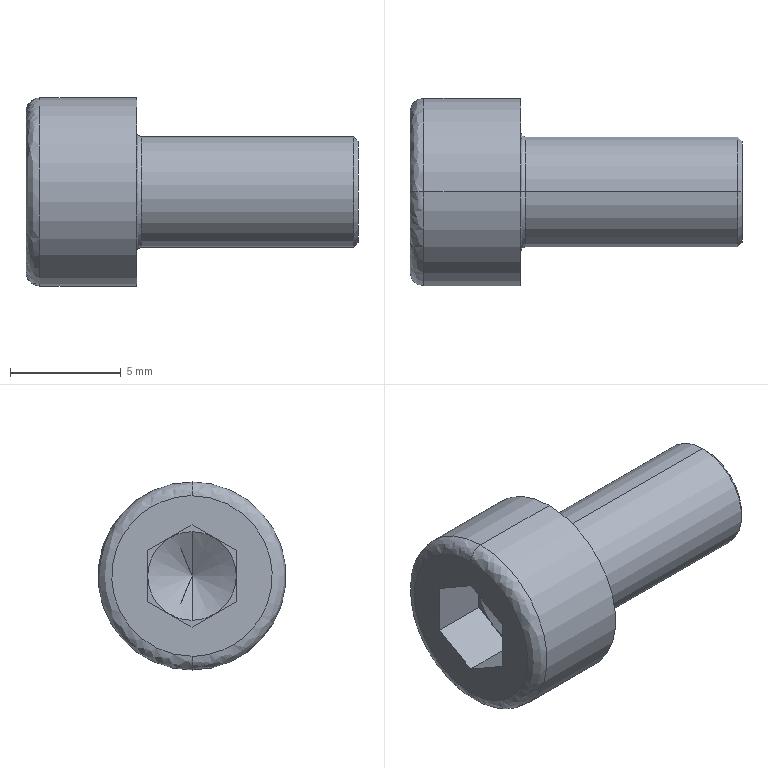Part | SolidWorks | features BaseBody 1 | 1 solid | 27 faces | box 15 x 8.5 x 8.5 mm | volume 438.278 mm3 | plane 15 | spline 4 | cylinder 4 | cone 4 | commonest cylinder face diameters 5 x2 8.5 x2
STEP:
#1=CARTESIAN_POINT('',(5.,0.,2.7));
#2=VERTEX_POINT('',#1);
#3=CARTESIAN_POINT('',(5.,0.,-2.7));
#4=VERTEX_POINT('',#3);
#5=CARTESIAN_POINT('',(5.,0.,2.7));
#6=CARTESIAN_POINT('',(5.,0.1716,2.7));
#7=CARTESIAN_POINT('',(5.,0.4245,2.676));
#8=CARTESIAN_POINT('',(5.,0.7118,2.607));
#9=CARTESIAN_POINT('',(5.,0.8535,2.562));
#10=CARTESIAN_POINT('',(5.,0.9138,2.541));
#11=CARTESIAN_POINT('',(5.,0.9539,2.526));
#12=CARTESIAN_POINT('',(5.,0.9722,2.519));
#13=CARTESIAN_POINT('',(5.,1.34,2.373));
#14=CARTESIAN_POINT('',(5.,1.646,2.172));
#15=CARTESIAN_POINT('',(5.,2.041,1.778));
#16=CARTESIAN_POINT('',(5.,2.215,1.564));
#17=CARTESIAN_POINT('',(5.,2.376,1.288));
#18=CARTESIAN_POINT('',(5.,2.447,1.143));
#19=CARTESIAN_POINT('',(5.,2.475,1.08));
#20=CARTESIAN_POINT('',(5.,2.493,1.037));
#21=CARTESIAN_POINT('',(5.,2.503,1.014));
#22=CARTESIAN_POINT('',(5.,2.637,0.675));
#23=CARTESIAN_POINT('',(5.,2.7,0.343));
#24=CARTESIAN_POINT('',(5.,2.7,-0.1715));
#25=CARTESIAN_POINT('',(5.,2.676,-0.4243));
#26=CARTESIAN_POINT('',(5.,2.607,-0.7117));
#27=CARTESIAN_POINT('',(5.,2.562,-0.8534));
#28=CARTESIAN_POINT('',(5.,2.541,-0.9137));
#29=CARTESIAN_POINT('',(5.,2.526,-0.9539));
#30=CARTESIAN_POINT('',(5.,2.519,-0.9722));
#31=CARTESIAN_POINT('',(5.,2.373,-1.34));
#32=CARTESIAN_POINT('',(5.,2.172,-1.646));
#33=CARTESIAN_POINT('',(5.,1.778,-2.041));
#34=CARTESIAN_POINT('',(5.,1.564,-2.215));
#35=CARTESIAN_POINT('',(5.,1.288,-2.376));
#36=CARTESIAN_POINT('',(5.,1.143,-2.447));
#37=CARTESIAN_POINT('',(5.,1.08,-2.475));
#38=CARTESIAN_POINT('',(5.,1.037,-2.493));
#39=CARTESIAN_POINT('',(5.,1.014,-2.503));
#40=CARTESIAN_POINT('',(5.,0.6748,-2.637));
#41=CARTESIAN_POINT('',(5.,0.3435,-2.7));
#42=CARTESIAN_POINT('',(5.,0.,-2.7));
#43=B_SPLINE_CURVE_WITH_KNOTS('',3,(#5,#6,#7,#8,#9,#10,#11,#12,#13,#14,#15,#16,#17,#18,#19,#20,#21,#22,#23,#24,#25,#26,#27,#28,#29,#30,#31,#32,#33,#34,#35,#36,#37,#38,#39,#40,#41,#42),.UNSPECIFIED.,.F.,.F.,(4,1,1,1,2,2,2,1,1,1,2,2,2,1,1,1,2,2,2,1,1,1,2,2,4),(0.,0.0625,0.09375,0.1094,0.1172,0.125,0.25,0.3125,0.3437,0.3594,0.3672,0.375,0.5,0.5625,0.5937,0.6094,0.6172,0.625,0.75,0.8125,0.8437,0.8594,0.8672,0.875,1.),.UNSPECIFIED.);
#44=EDGE_CURVE('',#2,#4,#43,.T.);
#45=ORIENTED_EDGE('',*,*,#44,.F.);
#46=CARTESIAN_POINT('',(5.2,0.,2.5));
#47=VERTEX_POINT('',#46);
#48=CARTESIAN_POINT('',(5.2,0.,2.7));
#49=DIRECTION('',(0.,-1.,0.));
#50=DIRECTION('',(0.,0.,1.));
#51=AXIS2_PLACEMENT_3D('',#48,#49,#50);
#52=CIRCLE('',#51,0.2);
#53=EDGE_CURVE('',#2,#47,#52,.T.);
#54=ORIENTED_EDGE('',*,*,#53,.T.);
#55=CARTESIAN_POINT('',(5.2,0.,-2.5));
#56=VERTEX_POINT('',#55);
#57=CARTESIAN_POINT('',(5.2,0.,0.));
#58=DIRECTION('',(1.,0.,0.));
#59=DIRECTION('',(0.,0.,1.));
#60=AXIS2_PLACEMENT_3D('',#57,#58,#59);
#61=CIRCLE('',#60,2.5);
#62=EDGE_CURVE('',#56,#47,#61,.T.);
#63=ORIENTED_EDGE('',*,*,#62,.F.);
#64=CARTESIAN_POINT('',(5.2,0.,-2.7));
#65=DIRECTION('',(0.,1.,0.));
#66=DIRECTION('',(0.,0.,-1.));
#67=AXIS2_PLACEMENT_3D('',#64,#65,#66);
#68=CIRCLE('',#67,0.2);
#69=EDGE_CURVE('',#4,#56,#68,.T.);
#70=ORIENTED_EDGE('',*,*,#69,.F.);
#71=EDGE_LOOP('',(#45,#54,#63,#70));
#72=FACE_OUTER_BOUND('',#71,.T.);
#73=CARTESIAN_POINT('',(5.,0.,-2.7));
#74=CARTESIAN_POINT('',(5.,5.4,-2.7));
#75=CARTESIAN_POINT('',(5.,5.4,2.7));
#76=CARTESIAN_POINT('',(5.,0.,2.7));
#77=CARTESIAN_POINT('',(5.,0.,-2.583));
#78=CARTESIAN_POINT('',(5.,5.166,-2.583));
#79=CARTESIAN_POINT('',(5.,5.166,2.583));
#80=CARTESIAN_POINT('',(5.,0.,2.583));
#81=CARTESIAN_POINT('',(5.083,0.,-2.5));
#82=CARTESIAN_POINT('',(5.083,5.,-2.5));
#83=CARTESIAN_POINT('',(5.083,5.,2.5));
#84=CARTESIAN_POINT('',(5.083,0.,2.5));
#85=CARTESIAN_POINT('',(5.2,0.,-2.5));
#86=CARTESIAN_POINT('',(5.2,5.,-2.5));
#87=CARTESIAN_POINT('',(5.2,5.,2.5));
#88=CARTESIAN_POINT('',(5.2,0.,2.5));
#89=(BOUNDED_SURFACE()B_SPLINE_SURFACE(3,3,((#73,#74,#75,#76),(#77,#78,#79,#80),(#81,#82,#83,#84),(#85,#86,#87,#88)),.UNSPECIFIED.,.F.,.F.,.F.)B_SPLINE_SURFACE_WITH_KNOTS((4,4),(4,4),(0.,1.),(0.,1.),.UNSPECIFIED.)GEOMETRIC_REPRESENTATION_ITEM()RATIONAL_B_SPLINE_SURFACE(((1.,0.3333,0.3333,1.),(0.8047,0.2682,0.2682,0.8047),(0.8047,0.2682,0.2682,0.8047),(1.,0.3333,0.3333,1.)))REPRESENTATION_ITEM('')SURFACE());
#90=ADVANCED_FACE('',(#72),#89,.F.);
#91=CARTESIAN_POINT('',(0.625,0.,4.25));
#92=VERTEX_POINT('',#91);
#93=CARTESIAN_POINT('',(0.625,0.,-4.25));
#94=VERTEX_POINT('',#93);
#95=CARTESIAN_POINT('',(0.625,0.,0.));
#96=DIRECTION('',(1.,0.,0.));
#97=DIRECTION('',(0.,0.,1.));
#98=AXIS2_PLACEMENT_3D('',#95,#96,#97);
#99=CIRCLE('',#98,4.25);
#100=EDGE_CURVE('',#92,#94,#99,.T.);
#101=ORIENTED_EDGE('',*,*,#100,.F.);
#102=CARTESIAN_POINT('',(0.,0.,3.625));
#103=VERTEX_POINT('',#102);
#104=CARTESIAN_POINT('',(0.625,0.,3.625));
#105=DIRECTION('',(0.,-1.,0.));
#106=DIRECTION('',(0.,0.,1.));
#107=AXIS2_PLACEMENT_3D('',#104,#105,#106);
#108=CIRCLE('',#107,0.625);
#109=EDGE_CURVE('',#92,#103,#108,.T.);
#110=ORIENTED_EDGE('',*,*,#109,.T.);
#111=CARTESIAN_POINT('',(0.,0.,-3.625));
#112=VERTEX_POINT('',#111);
#113=CARTESIAN_POINT('',(0.,0.,3.625));
#114=CARTESIAN_POINT('',(0.,-7.25,3.625));
#115=CARTESIAN_POINT('',(0.,-7.25,-3.625));
#116=CARTESIAN_POINT('',(0.,0.,-3.625));
#117=(BOUNDED_CURVE()B_SPLINE_CURVE(3,(#113,#114,#115,#116),.UNSPECIFIED.,.F.,.F.)B_SPLINE_CURVE_WITH_KNOTS((4,4),(0.,1.),.UNSPECIFIED.)CURVE()GEOMETRIC_REPRESENTATION_ITEM()RATIONAL_B_SPLINE_CURVE((1.,0.3333,0.3333,1.))REPRESENTATION_ITEM(''));
#118=EDGE_CURVE('',#103,#112,#117,.T.);
#119=ORIENTED_EDGE('',*,*,#118,.T.);
#120=CARTESIAN_POINT('',(0.625,0.,-3.625));
#121=DIRECTION('',(0.,1.,0.));
#122=DIRECTION('',(0.,0.,-1.));
#123=AXIS2_PLACEMENT_3D('',#120,#121,#122);
#124=CIRCLE('',#123,0.625);
#125=EDGE_CURVE('',#94,#112,#124,.T.);
#126=ORIENTED_EDGE('',*,*,#125,.F.);
#127=EDGE_LOOP('',(#101,#110,#119,#126));
#128=FACE_OUTER_BOUND('',#127,.T.);
#129=CARTESIAN_POINT('',(0.625,0.,4.25));
#130=CARTESIAN_POINT('',(0.625,-8.5,4.25));
#131=CARTESIAN_POINT('',(0.625,-8.5,-4.25));
#132=CARTESIAN_POINT('',(0.625,0.,-4.25));
#133=CARTESIAN_POINT('',(0.2589,0.,4.25));
#134=CARTESIAN_POINT('',(0.2589,-8.5,4.25));
#135=CARTESIAN_POINT('',(0.2589,-8.5,-4.25));
#136=CARTESIAN_POINT('',(0.2589,0.,-4.25));
#137=CARTESIAN_POINT('',(0.,0.,3.991));
#138=CARTESIAN_POINT('',(0.,-7.982,3.991));
#139=CARTESIAN_POINT('',(0.,-7.982,-3.991));
#140=CARTESIAN_POINT('',(0.,0.,-3.991));
#141=CARTESIAN_POINT('',(0.,0.,3.625));
#142=CARTESIAN_POINT('',(0.,-7.25,3.625));
#143=CARTESIAN_POINT('',(0.,-7.25,-3.625));
#144=CARTESIAN_POINT('',(0.,0.,-3.625));
#145=(BOUNDED_SURFACE()B_SPLINE_SURFACE(3,3,((#129,#130,#131,#132),(#133,#134,#135,#136),(#137,#138,#139,#140),(#141,#142,#143,#144)),.UNSPECIFIED.,.F.,.F.,.F.)B_SPLINE_SURFACE_WITH_KNOTS((4,4),(4,4),(0.,1.),(0.,1.),.UNSPECIFIED.)GEOMETRIC_REPRESENTATION_ITEM()RATIONAL_B_SPLINE_SURFACE(((1.,0.3333,0.3333,1.),(0.8047,0.2682,0.2682,0.8047),(0.8047,0.2682,0.2682,0.8047),(1.,0.3333,0.3333,1.)))REPRESENTATION_ITEM('')SURFACE());
#146=ADVANCED_FACE('',(#128),#145,.T.);
#147=CARTESIAN_POINT('',(14.8,0.,2.5));
#148=VERTEX_POINT('',#147);
#149=CARTESIAN_POINT('',(14.8,0.,-2.5));
#150=VERTEX_POINT('',#149);
#151=CARTESIAN_POINT('',(14.8,0.,0.));
#152=DIRECTION('',(-1.,0.,0.));
#153=DIRECTION('',(0.,0.,1.));
#154=AXIS2_PLACEMENT_3D('',#151,#152,#153);
#155=CIRCLE('',#154,2.5);
#156=EDGE_CURVE('',#148,#150,#155,.T.);
#157=ORIENTED_EDGE('',*,*,#156,.T.);
#158=CARTESIAN_POINT('',(15.,0.,-2.5));
#159=DIRECTION('',(-1.,0.,0.));
#160=VECTOR('',#159,1000.);
#161=LINE('',#158,#160);
#162=EDGE_CURVE('',#150,#56,#161,.T.);
#163=ORIENTED_EDGE('',*,*,#162,.T.);
#164=ORIENTED_EDGE('',*,*,#62,.T.);
#165=CARTESIAN_POINT('',(15.,0.,2.5));
#166=DIRECTION('',(-1.,0.,0.));
#167=VECTOR('',#166,1000.);
#168=LINE('',#165,#167);
#169=EDGE_CURVE('',#148,#47,#168,.T.);
#170=ORIENTED_EDGE('',*,*,#169,.F.);
#171=EDGE_LOOP('',(#157,#163,#164,#170));
#172=FACE_OUTER_BOUND('',#171,.T.);
#173=CARTESIAN_POINT('',(15.,0.,0.));
#174=DIRECTION('',(-1.,0.,0.));
#175=DIRECTION('',(0.,0.,1.));
#176=AXIS2_PLACEMENT_3D('',#173,#174,#175);
#177=CYLINDRICAL_SURFACE('',#176,2.5);
#178=ADVANCED_FACE('',(#172),#177,.T.);
#179=CARTESIAN_POINT('',(15.,0.,2.3));
#180=VERTEX_POINT('',#179);
#181=CARTESIAN_POINT('',(15.,0.,-2.3));
#182=VERTEX_POINT('',#181);
#183=CARTESIAN_POINT('',(15.,0.,0.));
#184=DIRECTION('',(-1.,0.,0.));
#185=DIRECTION('',(0.,0.,1.));
#186=AXIS2_PLACEMENT_3D('',#183,#184,#185);
#187=CIRCLE('',#186,2.3);
#188=EDGE_CURVE('',#180,#182,#187,.T.);
#189=ORIENTED_EDGE('',*,*,#188,.T.);
#190=CARTESIAN_POINT('',(14.8,0.,-2.5));
#191=DIRECTION('',(-0.7071,0.,-0.7071));
#192=VECTOR('',#191,1000.);
#193=LINE('',#190,#192);
#194=EDGE_CURVE('',#182,#150,#193,.T.);
#195=ORIENTED_EDGE('',*,*,#194,.T.);
#196=ORIENTED_EDGE('',*,*,#156,.F.);
#197=CARTESIAN_POINT('',(14.8,0.,2.5));
#198=DIRECTION('',(-0.7071,0.,0.7071));
#199=VECTOR('',#198,1000.);
#200=LINE('',#197,#199);
#201=EDGE_CURVE('',#180,#148,#200,.T.);
#202=ORIENTED_EDGE('',*,*,#201,.F.);
#203=EDGE_LOOP('',(#189,#195,#196,#202));
#204=FACE_OUTER_BOUND('',#203,.T.);
#205=CARTESIAN_POINT('',(14.8,0.,0.));
#206=DIRECTION('',(-1.,0.,0.));
#207=DIRECTION('',(0.,0.,1.));
#208=AXIS2_PLACEMENT_3D('',#205,#206,#207);
#209=CONICAL_SURFACE('',#208,2.5,0.7854);
#210=ADVANCED_FACE('',(#204),#209,.T.);
#211=CARTESIAN_POINT('',(5.,0.,-4.25));
#212=VERTEX_POINT('',#211);
#213=CARTESIAN_POINT('',(5.,0.,4.25));
#214=VERTEX_POINT('',#213);
#215=CARTESIAN_POINT('',(5.,0.,0.));
#216=DIRECTION('',(1.,0.,0.));
#217=DIRECTION('',(0.,0.,1.));
#218=AXIS2_PLACEMENT_3D('',#215,#216,#217);
#219=CIRCLE('',#218,4.25);
#220=EDGE_CURVE('',#212,#214,#219,.T.);
#221=ORIENTED_EDGE('',*,*,#220,.F.);
#222=CARTESIAN_POINT('',(5.,0.,-4.25));
#223=DIRECTION('',(-1.,0.,0.));
#224=VECTOR('',#223,1000.);
#225=LINE('',#222,#224);
#226=EDGE_CURVE('',#212,#94,#225,.T.);
#227=ORIENTED_EDGE('',*,*,#226,.T.);
#228=CARTESIAN_POINT('',(0.625,0.,0.));
#229=DIRECTION('',(1.,0.,0.));
#230=DIRECTION('',(0.,0.,1.));
#231=AXIS2_PLACEMENT_3D('',#228,#229,#230);
#232=CIRCLE('',#231,4.25);
#233=EDGE_CURVE('',#94,#92,#232,.T.);
#234=ORIENTED_EDGE('',*,*,#233,.T.);
#235=CARTESIAN_POINT('',(5.,0.,4.25));
#236=DIRECTION('',(-1.,0.,0.));
#237=VECTOR('',#236,1000.);
#238=LINE('',#235,#237);
#239=EDGE_CURVE('',#214,#92,#238,.T.);
#240=ORIENTED_EDGE('',*,*,#239,.F.);
#241=EDGE_LOOP('',(#221,#227,#234,#240));
#242=FACE_OUTER_BOUND('',#241,.T.);
#243=CARTESIAN_POINT('',(5.,0.,0.));
#244=DIRECTION('',(-1.,0.,0.));
#245=DIRECTION('',(0.,0.,1.));
#246=AXIS2_PLACEMENT_3D('',#243,#244,#245);
#247=CYLINDRICAL_SURFACE('',#246,4.25);
#248=ADVANCED_FACE('',(#242),#247,.T.);
#249=CARTESIAN_POINT('',(3.655,0.,0.));
#250=VERTEX_POINT('',#249);
#251=CARTESIAN_POINT('',(2.5,0.,2.));
#252=VERTEX_POINT('',#251);
#253=CARTESIAN_POINT('',(2.5,0.,2.));
#254=DIRECTION('',(-0.5,0.,0.866));
#255=VECTOR('',#254,1000.);
#256=LINE('',#253,#255);
#257=EDGE_CURVE('',#250,#252,#256,.T.);
#258=ORIENTED_EDGE('',*,*,#257,.F.);
#259=CARTESIAN_POINT('',(2.5,0.,-2.));
#260=VERTEX_POINT('',#259);
#261=CARTESIAN_POINT('',(2.5,0.,-2.));
#262=DIRECTION('',(-0.5,0.,-0.866));
#263=VECTOR('',#262,1000.);
#264=LINE('',#261,#263);
#265=EDGE_CURVE('',#250,#260,#264,.T.);
#266=ORIENTED_EDGE('',*,*,#265,.T.);
#267=CARTESIAN_POINT('',(2.5,-1.,-1.732));
#268=VERTEX_POINT('',#267);
#269=CARTESIAN_POINT('',(2.5,0.,0.));
#270=DIRECTION('',(1.,0.,0.));
#271=DIRECTION('',(0.,0.,1.));
#272=AXIS2_PLACEMENT_3D('',#269,#270,#271);
#273=CIRCLE('',#272,2.);
#274=EDGE_CURVE('',#268,#260,#273,.T.);
#275=ORIENTED_EDGE('',*,*,#274,.F.);
#276=CARTESIAN_POINT('',(2.5,-2.,0.));
#277=VERTEX_POINT('',#276);
#278=CARTESIAN_POINT('',(2.5,0.,0.));
#279=DIRECTION('',(-1.,0.,0.));
#280=DIRECTION('',(0.,0.,1.));
#281=AXIS2_PLACEMENT_3D('',#278,#279,#280);
#282=CIRCLE('',#281,2.);
#283=EDGE_CURVE('',#268,#277,#282,.T.);
#284=ORIENTED_EDGE('',*,*,#283,.T.);
#285=CARTESIAN_POINT('',(2.5,-1.,1.732));
#286=VERTEX_POINT('',#285);
#287=CARTESIAN_POINT('',(2.5,0.,0.));
#288=DIRECTION('',(1.,0.,0.));
#289=DIRECTION('',(0.,0.,1.));
#290=AXIS2_PLACEMENT_3D('',#287,#288,#289);
#291=CIRCLE('',#290,2.);
#292=EDGE_CURVE('',#286,#277,#291,.T.);
#293=ORIENTED_EDGE('',*,*,#292,.F.);
#294=CARTESIAN_POINT('',(2.5,0.,0.));
#295=DIRECTION('',(1.,0.,0.));
#296=DIRECTION('',(0.,0.,1.));
#297=AXIS2_PLACEMENT_3D('',#294,#295,#296);
#298=CIRCLE('',#297,2.);
#299=EDGE_CURVE('',#252,#286,#298,.T.);
#300=ORIENTED_EDGE('',*,*,#299,.F.);
#301=EDGE_LOOP('',(#258,#266,#275,#284,#293,#300));
#302=FACE_OUTER_BOUND('',#301,.T.);
#303=CARTESIAN_POINT('',(2.5,0.,0.));
#304=DIRECTION('',(-1.,0.,0.));
#305=DIRECTION('',(0.,0.,1.));
#306=AXIS2_PLACEMENT_3D('',#303,#304,#305);
#307=CONICAL_SURFACE('',#306,2.,1.047);
#308=ADVANCED_FACE('',(#302),#307,.F.);
#309=ORIENTED_EDGE('',*,*,#162,.F.);
#310=CARTESIAN_POINT('',(14.8,0.,0.));
#311=DIRECTION('',(-1.,0.,0.));
#312=DIRECTION('',(0.,0.,1.));
#313=AXIS2_PLACEMENT_3D('',#310,#311,#312);
#314=CIRCLE('',#313,2.5);
#315=EDGE_CURVE('',#150,#148,#314,.T.);
#316=ORIENTED_EDGE('',*,*,#315,.T.);
#317=ORIENTED_EDGE('',*,*,#169,.T.);
#318=CARTESIAN_POINT('',(5.2,0.,0.));
#319=DIRECTION('',(1.,0.,0.));
#320=DIRECTION('',(0.,0.,1.));
#321=AXIS2_PLACEMENT_3D('',#318,#319,#320);
#322=CIRCLE('',#321,2.5);
#323=EDGE_CURVE('',#47,#56,#322,.T.);
#324=ORIENTED_EDGE('',*,*,#323,.T.);
#325=EDGE_LOOP('',(#309,#316,#317,#324));
#326=FACE_OUTER_BOUND('',#325,.T.);
#327=CARTESIAN_POINT('',(15.,0.,0.));
#328=DIRECTION('',(-1.,0.,0.));
#329=DIRECTION('',(0.,0.,1.));
#330=AXIS2_PLACEMENT_3D('',#327,#328,#329);
#331=CYLINDRICAL_SURFACE('',#330,2.5);
#332=ADVANCED_FACE('',(#326),#331,.T.);
#333=ORIENTED_EDGE('',*,*,#53,.F.);
#334=CARTESIAN_POINT('',(5.,0.,-2.7));
#335=CARTESIAN_POINT('',(5.,-0.1716,-2.7));
#336=CARTESIAN_POINT('',(5.,-0.4245,-2.676));
#337=CARTESIAN_POINT('',(5.,-0.7118,-2.607));
#338=CARTESIAN_POINT('',(5.,-0.8535,-2.562));
#339=CARTESIAN_POINT('',(5.,-0.9138,-2.541));
#340=CARTESIAN_POINT('',(5.,-0.9539,-2.526));
#341=CARTESIAN_POINT('',(5.,-0.9722,-2.519));
#342=CARTESIAN_POINT('',(5.,-1.34,-2.373));
#343=CARTESIAN_POINT('',(5.,-1.646,-2.172));
#344=CARTESIAN_POINT('',(5.,-2.041,-1.778));
#345=CARTESIAN_POINT('',(5.,-2.215,-1.564));
#346=CARTESIAN_POINT('',(5.,-2.376,-1.288));
#347=CARTESIAN_POINT('',(5.,-2.447,-1.143));
#348=CARTESIAN_POINT('',(5.,-2.475,-1.08));
#349=CARTESIAN_POINT('',(5.,-2.493,-1.037));
#350=CARTESIAN_POINT('',(5.,-2.503,-1.014));
#351=CARTESIAN_POINT('',(5.,-2.637,-0.675));
#352=CARTESIAN_POINT('',(5.,-2.7,-0.343));
#353=CARTESIAN_POINT('',(5.,-2.7,0.1715));
#354=CARTESIAN_POINT('',(5.,-2.676,0.4243));
#355=CARTESIAN_POINT('',(5.,-2.607,0.7117));
#356=CARTESIAN_POINT('',(5.,-2.562,0.8534));
#357=CARTESIAN_POINT('',(5.,-2.541,0.9137));
#358=CARTESIAN_POINT('',(5.,-2.526,0.9539));
#359=CARTESIAN_POINT('',(5.,-2.519,0.9722));
#360=CARTESIAN_POINT('',(5.,-2.373,1.34));
#361=CARTESIAN_POINT('',(5.,-2.172,1.646));
#362=CARTESIAN_POINT('',(5.,-1.778,2.041));
#363=CARTESIAN_POINT('',(5.,-1.564,2.215));
#364=CARTESIAN_POINT('',(5.,-1.288,2.376));
#365=CARTESIAN_POINT('',(5.,-1.143,2.447));
#366=CARTESIAN_POINT('',(5.,-1.08,2.475));
#367=CARTESIAN_POINT('',(5.,-1.037,2.493));
#368=CARTESIAN_POINT('',(5.,-1.014,2.503));
#369=CARTESIAN_POINT('',(5.,-0.6748,2.637));
#370=CARTESIAN_POINT('',(5.,-0.3435,2.7));
#371=CARTESIAN_POINT('',(5.,0.,2.7));
#372=B_SPLINE_CURVE_WITH_KNOTS('',3,(#334,#335,#336,#337,#338,#339,#340,#341,#342,#343,#344,#345,#346,#347,#348,#349,#350,#351,#352,#353,#354,#355,#356,#357,#358,#359,#360,#361,#362,#363,#364,#365,#366,#367,#368,#369,#370,#371),.UNSPECIFIED.,.F.,.F.,(4,1,1,1,2,2,2,1,1,1,2,2,2,1,1,1,2,2,2,1,1,1,2,2,4),(0.,0.0625,0.09375,0.1094,0.1172,0.125,0.25,0.3125,0.3437,0.3594,0.3672,0.375,0.5,0.5625,0.5937,0.6094,0.6172,0.625,0.75,0.8125,0.8437,0.8594,0.8672,0.875,1.),.UNSPECIFIED.);
#373=EDGE_CURVE('',#4,#2,#372,.T.);
#374=ORIENTED_EDGE('',*,*,#373,.F.);
#375=ORIENTED_EDGE('',*,*,#69,.T.);
#376=ORIENTED_EDGE('',*,*,#323,.F.);
#377=EDGE_LOOP('',(#333,#374,#375,#376));
#378=FACE_OUTER_BOUND('',#377,.T.);
#379=CARTESIAN_POINT('',(5.,0.,2.7));
#380=CARTESIAN_POINT('',(5.,-5.4,2.7));
#381=CARTESIAN_POINT('',(5.,-5.4,-2.7));
#382=CARTESIAN_POINT('',(5.,0.,-2.7));
#383=CARTESIAN_POINT('',(5.,0.,2.583));
#384=CARTESIAN_POINT('',(5.,-5.166,2.583));
#385=CARTESIAN_POINT('',(5.,-5.166,-2.583));
#386=CARTESIAN_POINT('',(5.,0.,-2.583));
#387=CARTESIAN_POINT('',(5.083,0.,2.5));
#388=CARTESIAN_POINT('',(5.083,-5.,2.5));
#389=CARTESIAN_POINT('',(5.083,-5.,-2.5));
#390=CARTESIAN_POINT('',(5.083,0.,-2.5));
#391=CARTESIAN_POINT('',(5.2,0.,2.5));
#392=CARTESIAN_POINT('',(5.2,-5.,2.5));
#393=CARTESIAN_POINT('',(5.2,-5.,-2.5));
#394=CARTESIAN_POINT('',(5.2,0.,-2.5));
#395=(BOUNDED_SURFACE()B_SPLINE_SURFACE(3,3,((#379,#380,#381,#382),(#383,#384,#385,#386),(#387,#388,#389,#390),(#391,#392,#393,#394)),.UNSPECIFIED.,.F.,.F.,.F.)B_SPLINE_SURFACE_WITH_KNOTS((4,4),(4,4),(0.,1.),(0.,1.),.UNSPECIFIED.)GEOMETRIC_REPRESENTATION_ITEM()RATIONAL_B_SPLINE_SURFACE(((1.,0.3333,0.3333,1.),(0.8047,0.2682,0.2682,0.8047),(0.8047,0.2682,0.2682,0.8047),(1.,0.3333,0.3333,1.)))REPRESENTATION_ITEM('')SURFACE());
#396=ADVANCED_FACE('',(#378),#395,.F.);
#397=ORIENTED_EDGE('',*,*,#194,.F.);
#398=CARTESIAN_POINT('',(15.,0.,0.));
#399=DIRECTION('',(-1.,0.,0.));
#400=DIRECTION('',(0.,0.,1.));
#401=AXIS2_PLACEMENT_3D('',#398,#399,#400);
#402=CIRCLE('',#401,2.3);
#403=EDGE_CURVE('',#182,#180,#402,.T.);
#404=ORIENTED_EDGE('',*,*,#403,.T.);
#405=ORIENTED_EDGE('',*,*,#201,.T.);
#406=ORIENTED_EDGE('',*,*,#315,.F.);
#407=EDGE_LOOP('',(#397,#404,#405,#406));
#408=FACE_OUTER_BOUND('',#407,.T.);
#409=CARTESIAN_POINT('',(14.8,0.,0.));
#410=DIRECTION('',(-1.,0.,0.));
#411=DIRECTION('',(0.,0.,1.));
#412=AXIS2_PLACEMENT_3D('',#409,#410,#411);
#413=CONICAL_SURFACE('',#412,2.5,0.7854);
#414=ADVANCED_FACE('',(#408),#413,.T.);
#415=CARTESIAN_POINT('',(5.,0.,0.));
#416=DIRECTION('',(1.,0.,0.));
#417=DIRECTION('',(0.,0.,1.));
#418=AXIS2_PLACEMENT_3D('',#415,#416,#417);
#419=CIRCLE('',#418,4.25);
#420=EDGE_CURVE('',#214,#212,#419,.T.);
#421=ORIENTED_EDGE('',*,*,#420,.T.);
#422=ORIENTED_EDGE('',*,*,#220,.T.);
#423=EDGE_LOOP('',(#421,#422));
#424=FACE_OUTER_BOUND('',#423,.T.);
#425=ORIENTED_EDGE('',*,*,#373,.T.);
#426=ORIENTED_EDGE('',*,*,#44,.T.);
#427=EDGE_LOOP('',(#425,#426));
#428=FACE_BOUND('',#427,.T.);
#429=CARTESIAN_POINT('',(5.,0.,0.));
#430=DIRECTION('',(1.,0.,0.));
#431=DIRECTION('',(0.,0.,-1.));
#432=AXIS2_PLACEMENT_3D('',#429,#430,#431);
#433=PLANE('',#432);
#434=ADVANCED_FACE('',(#424,#428),#433,.T.);
#435=ORIENTED_EDGE('',*,*,#188,.F.);
#436=ORIENTED_EDGE('',*,*,#403,.F.);
#437=EDGE_LOOP('',(#435,#436));
#438=FACE_OUTER_BOUND('',#437,.T.);
#439=CARTESIAN_POINT('',(15.,0.,0.));
#440=DIRECTION('',(1.,0.,0.));
#441=DIRECTION('',(0.,0.,-1.));
#442=AXIS2_PLACEMENT_3D('',#439,#440,#441);
#443=PLANE('',#442);
#444=ADVANCED_FACE('',(#438),#443,.T.);
#445=ORIENTED_EDGE('',*,*,#226,.F.);
#446=ORIENTED_EDGE('',*,*,#420,.F.);
#447=ORIENTED_EDGE('',*,*,#239,.T.);
#448=ORIENTED_EDGE('',*,*,#100,.T.);
#449=EDGE_LOOP('',(#445,#446,#447,#448));
#450=FACE_OUTER_BOUND('',#449,.T.);
#451=CARTESIAN_POINT('',(5.,0.,0.));
#452=DIRECTION('',(-1.,0.,0.));
#453=DIRECTION('',(0.,0.,1.));
#454=AXIS2_PLACEMENT_3D('',#451,#452,#453);
#455=CYLINDRICAL_SURFACE('',#454,4.25);
#456=ADVANCED_FACE('',(#450),#455,.T.);
#457=ORIENTED_EDGE('',*,*,#109,.F.);
#458=ORIENTED_EDGE('',*,*,#233,.F.);
#459=ORIENTED_EDGE('',*,*,#125,.T.);
#460=CARTESIAN_POINT('',(0.,0.,-3.625));
#461=CARTESIAN_POINT('',(0.,7.25,-3.625));
#462=CARTESIAN_POINT('',(0.,7.25,3.625));
#463=CARTESIAN_POINT('',(0.,0.,3.625));
#464=(BOUNDED_CURVE()B_SPLINE_CURVE(3,(#460,#461,#462,#463),.UNSPECIFIED.,.F.,.T.)B_SPLINE_CURVE_WITH_KNOTS((4,4),(0.,1.),.UNSPECIFIED.)CURVE()GEOMETRIC_REPRESENTATION_ITEM()RATIONAL_B_SPLINE_CURVE((1.,0.3333,0.3333,1.))REPRESENTATION_ITEM(''));
#465=EDGE_CURVE('',#112,#103,#464,.T.);
#466=ORIENTED_EDGE('',*,*,#465,.T.);
#467=EDGE_LOOP('',(#457,#458,#459,#466));
#468=FACE_OUTER_BOUND('',#467,.T.);
#469=CARTESIAN_POINT('',(0.625,0.,-4.25));
#470=CARTESIAN_POINT('',(0.625,8.5,-4.25));
#471=CARTESIAN_POINT('',(0.625,8.5,4.25));
#472=CARTESIAN_POINT('',(0.625,0.,4.25));
#473=CARTESIAN_POINT('',(0.2589,0.,-4.25));
#474=CARTESIAN_POINT('',(0.2589,8.5,-4.25));
#475=CARTESIAN_POINT('',(0.2589,8.5,4.25));
#476=CARTESIAN_POINT('',(0.2589,0.,4.25));
#477=CARTESIAN_POINT('',(0.,0.,-3.991));
#478=CARTESIAN_POINT('',(0.,7.982,-3.991));
#479=CARTESIAN_POINT('',(0.,7.982,3.991));
#480=CARTESIAN_POINT('',(0.,0.,3.991));
#481=CARTESIAN_POINT('',(0.,0.,-3.625));
#482=CARTESIAN_POINT('',(0.,7.25,-3.625));
#483=CARTESIAN_POINT('',(0.,7.25,3.625));
#484=CARTESIAN_POINT('',(0.,0.,3.625));
#485=(BOUNDED_SURFACE()B_SPLINE_SURFACE(3,3,((#469,#470,#471,#472),(#473,#474,#475,#476),(#477,#478,#479,#480),(#481,#482,#483,#484)),.UNSPECIFIED.,.F.,.F.,.F.)B_SPLINE_SURFACE_WITH_KNOTS((4,4),(4,4),(0.,1.),(0.,1.),.UNSPECIFIED.)GEOMETRIC_REPRESENTATION_ITEM()RATIONAL_B_SPLINE_SURFACE(((1.,0.3333,0.3333,1.),(0.8047,0.2682,0.2682,0.8047),(0.8047,0.2682,0.2682,0.8047),(1.,0.3333,0.3333,1.)))REPRESENTATION_ITEM('')SURFACE());
#486=ADVANCED_FACE('',(#468),#485,.T.);
#487=CARTESIAN_POINT('',(0.,2.,1.155));
#488=VERTEX_POINT('',#487);
#489=CARTESIAN_POINT('',(0.,2.,-1.155));
#490=VERTEX_POINT('',#489);
#491=CARTESIAN_POINT('',(0.,2.,0.));
#492=DIRECTION('',(0.,0.,-1.));
#493=VECTOR('',#492,1000.);
#494=LINE('',#491,#493);
#495=EDGE_CURVE('',#488,#490,#494,.T.);
#496=ORIENTED_EDGE('',*,*,#495,.F.);
#497=CARTESIAN_POINT('',(0.,0.,2.309));
#498=VERTEX_POINT('',#497);
#499=CARTESIAN_POINT('',(0.,0.,2.309));
#500=DIRECTION('',(0.,0.866,-0.5));
#501=VECTOR('',#500,1000.);
#502=LINE('',#499,#501);
#503=EDGE_CURVE('',#498,#488,#502,.T.);
#504=ORIENTED_EDGE('',*,*,#503,.F.);
#505=CARTESIAN_POINT('',(0.,-2.,1.155));
#506=VERTEX_POINT('',#505);
#507=CARTESIAN_POINT('',(0.,-2.,1.155));
#508=DIRECTION('',(0.,0.866,0.5));
#509=VECTOR('',#508,1000.);
#510=LINE('',#507,#509);
#511=EDGE_CURVE('',#506,#498,#510,.T.);
#512=ORIENTED_EDGE('',*,*,#511,.F.);
#513=CARTESIAN_POINT('',(0.,-2.,-1.155));
#514=VERTEX_POINT('',#513);
#515=CARTESIAN_POINT('',(0.,-2.,0.));
#516=DIRECTION('',(0.,0.,1.));
#517=VECTOR('',#516,1000.);
#518=LINE('',#515,#517);
#519=EDGE_CURVE('',#514,#506,#518,.T.);
#520=ORIENTED_EDGE('',*,*,#519,.F.);
#521=CARTESIAN_POINT('',(0.,0.,-2.309));
#522=VERTEX_POINT('',#521);
#523=CARTESIAN_POINT('',(0.,0.,-2.309));
#524=DIRECTION('',(0.,-0.866,0.5));
#525=VECTOR('',#524,1000.);
#526=LINE('',#523,#525);
#527=EDGE_CURVE('',#522,#514,#526,.T.);
#528=ORIENTED_EDGE('',*,*,#527,.F.);
#529=CARTESIAN_POINT('',(0.,2.,-1.155));
#530=DIRECTION('',(0.,-0.866,-0.5));
#531=VECTOR('',#530,1000.);
#532=LINE('',#529,#531);
#533=EDGE_CURVE('',#490,#522,#532,.T.);
#534=ORIENTED_EDGE('',*,*,#533,.F.);
#535=EDGE_LOOP('',(#496,#504,#512,#520,#528,#534));
#536=FACE_BOUND('',#535,.T.);
#537=ORIENTED_EDGE('',*,*,#465,.F.);
#538=ORIENTED_EDGE('',*,*,#118,.F.);
#539=EDGE_LOOP('',(#537,#538));
#540=FACE_OUTER_BOUND('',#539,.T.);
#541=CARTESIAN_POINT('',(0.,0.,0.));
#542=DIRECTION('',(1.,0.,0.));
#543=DIRECTION('',(0.,0.,-1.));
#544=AXIS2_PLACEMENT_3D('',#541,#542,#543);
#545=PLANE('',#544);
#546=ADVANCED_FACE('',(#536,#540),#545,.F.);
#547=CARTESIAN_POINT('',(2.5,0.,-2.309));
#548=VERTEX_POINT('',#547);
#549=CARTESIAN_POINT('',(2.5,0.,-2.309));
#550=DIRECTION('',(1.,0.,0.));
#551=VECTOR('',#550,1000.);
#552=LINE('',#549,#551);
#553=EDGE_CURVE('',#522,#548,#552,.T.);
#554=ORIENTED_EDGE('',*,*,#553,.T.);
#555=CARTESIAN_POINT('',(2.5,1.,-1.732));
#556=VERTEX_POINT('',#555);
#557=CARTESIAN_POINT('',(2.5,0.,-2.309));
#558=DIRECTION('',(0.,0.866,0.5));
#559=VECTOR('',#558,1000.);
#560=LINE('',#557,#559);
#561=EDGE_CURVE('',#548,#556,#560,.T.);
#562=ORIENTED_EDGE('',*,*,#561,.T.);
#563=CARTESIAN_POINT('',(2.5,2.,-1.155));
#564=VERTEX_POINT('',#563);
#565=CARTESIAN_POINT('',(2.5,1.,-1.732));
#566=DIRECTION('',(0.,0.866,0.5));
#567=VECTOR('',#566,1000.);
#568=LINE('',#565,#567);
#569=EDGE_CURVE('',#556,#564,#568,.T.);
#570=ORIENTED_EDGE('',*,*,#569,.T.);
#571=CARTESIAN_POINT('',(2.5,2.,-1.155));
#572=DIRECTION('',(-1.,0.,0.));
#573=VECTOR('',#572,1000.);
#574=LINE('',#571,#573);
#575=EDGE_CURVE('',#564,#490,#574,.T.);
#576=ORIENTED_EDGE('',*,*,#575,.T.);
#577=ORIENTED_EDGE('',*,*,#533,.T.);
#578=EDGE_LOOP('',(#554,#562,#570,#576,#577));
#579=FACE_OUTER_BOUND('',#578,.T.);
#580=CARTESIAN_POINT('',(2.5,0.,-2.309));
#581=DIRECTION('',(0.,-0.5,0.866));
#582=DIRECTION('',(0.,-0.866,-0.5));
#583=AXIS2_PLACEMENT_3D('',#580,#581,#582);
#584=PLANE('',#583);
#585=ADVANCED_FACE('',(#579),#584,.T.);
#586=ORIENTED_EDGE('',*,*,#575,.F.);
#587=CARTESIAN_POINT('',(2.5,2.,0.));
#588=VERTEX_POINT('',#587);
#589=CARTESIAN_POINT('',(2.5,2.,-2.309));
#590=DIRECTION('',(0.,0.,1.));
#591=VECTOR('',#590,1000.);
#592=LINE('',#589,#591);
#593=EDGE_CURVE('',#564,#588,#592,.T.);
#594=ORIENTED_EDGE('',*,*,#593,.T.);
#595=CARTESIAN_POINT('',(2.5,2.,1.155));
#596=VERTEX_POINT('',#595);
#597=CARTESIAN_POINT('',(2.5,2.,-2.309));
#598=DIRECTION('',(0.,0.,1.));
#599=VECTOR('',#598,1000.);
#600=LINE('',#597,#599);
#601=EDGE_CURVE('',#588,#596,#600,.T.);
#602=ORIENTED_EDGE('',*,*,#601,.T.);
#603=CARTESIAN_POINT('',(2.5,2.,1.155));
#604=DIRECTION('',(-1.,0.,0.));
#605=VECTOR('',#604,1000.);
#606=LINE('',#603,#605);
#607=EDGE_CURVE('',#596,#488,#606,.T.);
#608=ORIENTED_EDGE('',*,*,#607,.T.);
#609=ORIENTED_EDGE('',*,*,#495,.T.);
#610=EDGE_LOOP('',(#586,#594,#602,#608,#609));
#611=FACE_OUTER_BOUND('',#610,.T.);
#612=CARTESIAN_POINT('',(2.5,2.,-1.155));
#613=DIRECTION('',(0.,-1.,0.));
#614=DIRECTION('',(0.,0.,-1.));
#615=AXIS2_PLACEMENT_3D('',#612,#613,#614);
#616=PLANE('',#615);
#617=ADVANCED_FACE('',(#611),#616,.T.);
#618=ORIENTED_EDGE('',*,*,#607,.F.);
#619=CARTESIAN_POINT('',(2.5,1.,1.732));
#620=VERTEX_POINT('',#619);
#621=CARTESIAN_POINT('',(2.5,2.,1.155));
#622=DIRECTION('',(0.,-0.866,0.5));
#623=VECTOR('',#622,1000.);
#624=LINE('',#621,#623);
#625=EDGE_CURVE('',#596,#620,#624,.T.);
#626=ORIENTED_EDGE('',*,*,#625,.T.);
#627=CARTESIAN_POINT('',(2.5,0.,2.309));
#628=VERTEX_POINT('',#627);
#629=CARTESIAN_POINT('',(2.5,2.,1.155));
#630=DIRECTION('',(0.,-0.866,0.5));
#631=VECTOR('',#630,1000.);
#632=LINE('',#629,#631);
#633=EDGE_CURVE('',#620,#628,#632,.T.);
#634=ORIENTED_EDGE('',*,*,#633,.T.);
#635=CARTESIAN_POINT('',(2.5,0.,2.309));
#636=DIRECTION('',(-1.,0.,0.));
#637=VECTOR('',#636,1000.);
#638=LINE('',#635,#637);
#639=EDGE_CURVE('',#628,#498,#638,.T.);
#640=ORIENTED_EDGE('',*,*,#639,.T.);
#641=ORIENTED_EDGE('',*,*,#503,.T.);
#642=EDGE_LOOP('',(#618,#626,#634,#640,#641));
#643=FACE_OUTER_BOUND('',#642,.T.);
#644=CARTESIAN_POINT('',(2.5,2.,1.155));
#645=DIRECTION('',(0.,-0.5,-0.866));
#646=DIRECTION('',(0.,0.866,-0.5));
#647=AXIS2_PLACEMENT_3D('',#644,#645,#646);
#648=PLANE('',#647);
#649=ADVANCED_FACE('',(#643),#648,.T.);
#650=ORIENTED_EDGE('',*,*,#639,.F.);
#651=CARTESIAN_POINT('',(2.5,0.,2.309));
#652=DIRECTION('',(0.,-0.866,-0.5));
#653=VECTOR('',#652,1000.);
#654=LINE('',#651,#653);
#655=EDGE_CURVE('',#628,#286,#654,.T.);
#656=ORIENTED_EDGE('',*,*,#655,.T.);
#657=CARTESIAN_POINT('',(2.5,-2.,1.155));
#658=VERTEX_POINT('',#657);
#659=CARTESIAN_POINT('',(2.5,-1.,1.732));
#660=DIRECTION('',(0.,-0.866,-0.5));
#661=VECTOR('',#660,1000.);
#662=LINE('',#659,#661);
#663=EDGE_CURVE('',#286,#658,#662,.T.);
#664=ORIENTED_EDGE('',*,*,#663,.T.);
#665=CARTESIAN_POINT('',(2.5,-2.,1.155));
#666=DIRECTION('',(-1.,0.,0.));
#667=VECTOR('',#666,1000.);
#668=LINE('',#665,#667);
#669=EDGE_CURVE('',#658,#506,#668,.T.);
#670=ORIENTED_EDGE('',*,*,#669,.T.);
#671=ORIENTED_EDGE('',*,*,#511,.T.);
#672=EDGE_LOOP('',(#650,#656,#664,#670,#671));
#673=FACE_OUTER_BOUND('',#672,.T.);
#674=CARTESIAN_POINT('',(2.5,0.,2.309));
#675=DIRECTION('',(0.,0.5,-0.866));
#676=DIRECTION('',(0.,0.866,0.5));
#677=AXIS2_PLACEMENT_3D('',#674,#675,#676);
#678=PLANE('',#677);
#679=ADVANCED_FACE('',(#673),#678,.T.);
#680=ORIENTED_EDGE('',*,*,#669,.F.);
#681=CARTESIAN_POINT('',(2.5,-2.,-2.309));
#682=DIRECTION('',(0.,0.,-1.));
#683=VECTOR('',#682,1000.);
#684=LINE('',#681,#683);
#685=EDGE_CURVE('',#658,#277,#684,.T.);
#686=ORIENTED_EDGE('',*,*,#685,.T.);
#687=CARTESIAN_POINT('',(2.5,-2.,-1.155));
#688=VERTEX_POINT('',#687);
#689=CARTESIAN_POINT('',(2.5,-2.,1.155));
#690=DIRECTION('',(0.,0.,-1.));
#691=VECTOR('',#690,1000.);
#692=LINE('',#689,#691);
#693=EDGE_CURVE('',#277,#688,#692,.T.);
#694=ORIENTED_EDGE('',*,*,#693,.T.);
#695=CARTESIAN_POINT('',(2.5,-2.,-1.155));
#696=DIRECTION('',(-1.,0.,0.));
#697=VECTOR('',#696,1000.);
#698=LINE('',#695,#697);
#699=EDGE_CURVE('',#688,#514,#698,.T.);
#700=ORIENTED_EDGE('',*,*,#699,.T.);
#701=ORIENTED_EDGE('',*,*,#519,.T.);
#702=EDGE_LOOP('',(#680,#686,#694,#700,#701));
#703=FACE_OUTER_BOUND('',#702,.T.);
#704=CARTESIAN_POINT('',(2.5,-2.,1.155));
#705=DIRECTION('',(0.,1.,0.));
#706=DIRECTION('',(0.,0.,1.));
#707=AXIS2_PLACEMENT_3D('',#704,#705,#706);
#708=PLANE('',#707);
#709=ADVANCED_FACE('',(#703),#708,.T.);
#710=ORIENTED_EDGE('',*,*,#699,.F.);
#711=CARTESIAN_POINT('',(2.5,-2.,-1.155));
#712=DIRECTION('',(0.,0.866,-0.5));
#713=VECTOR('',#712,1000.);
#714=LINE('',#711,#713);
#715=EDGE_CURVE('',#688,#268,#714,.T.);
#716=ORIENTED_EDGE('',*,*,#715,.T.);
#717=CARTESIAN_POINT('',(2.5,-2.,-1.155));
#718=DIRECTION('',(0.,0.866,-0.5));
#719=VECTOR('',#718,1000.);
#720=LINE('',#717,#719);
#721=EDGE_CURVE('',#268,#548,#720,.T.);
#722=ORIENTED_EDGE('',*,*,#721,.T.);
#723=ORIENTED_EDGE('',*,*,#553,.F.);
#724=ORIENTED_EDGE('',*,*,#527,.T.);
#725=EDGE_LOOP('',(#710,#716,#722,#723,#724));
#726=FACE_OUTER_BOUND('',#725,.T.);
#727=CARTESIAN_POINT('',(2.5,-2.,-1.155));
#728=DIRECTION('',(0.,0.5,0.866));
#729=DIRECTION('',(0.,-0.866,0.5));
#730=AXIS2_PLACEMENT_3D('',#727,#728,#729);
#731=PLANE('',#730);
#732=ADVANCED_FACE('',(#726),#731,.T.);
#733=ORIENTED_EDGE('',*,*,#274,.T.);
#734=CARTESIAN_POINT('',(2.5,0.,0.));
#735=DIRECTION('',(1.,0.,0.));
#736=DIRECTION('',(0.,0.,1.));
#737=AXIS2_PLACEMENT_3D('',#734,#735,#736);
#738=CIRCLE('',#737,2.);
#739=EDGE_CURVE('',#260,#556,#738,.T.);
#740=ORIENTED_EDGE('',*,*,#739,.T.);
#741=ORIENTED_EDGE('',*,*,#561,.F.);
#742=ORIENTED_EDGE('',*,*,#721,.F.);
#743=EDGE_LOOP('',(#733,#740,#741,#742));
#744=FACE_OUTER_BOUND('',#743,.T.);
#745=CARTESIAN_POINT('',(2.5,0.,-2.309));
#746=DIRECTION('',(1.,0.,0.));
#747=DIRECTION('',(0.,0.,-1.));
#748=AXIS2_PLACEMENT_3D('',#745,#746,#747);
#749=PLANE('',#748);
#750=ADVANCED_FACE('',(#744),#749,.F.);
#751=ORIENTED_EDGE('',*,*,#633,.F.);
#752=CARTESIAN_POINT('',(2.5,0.,0.));
#753=DIRECTION('',(1.,0.,0.));
#754=DIRECTION('',(0.,0.,1.));
#755=AXIS2_PLACEMENT_3D('',#752,#753,#754);
#756=CIRCLE('',#755,2.);
#757=EDGE_CURVE('',#620,#252,#756,.T.);
#758=ORIENTED_EDGE('',*,*,#757,.T.);
#759=ORIENTED_EDGE('',*,*,#299,.T.);
#760=ORIENTED_EDGE('',*,*,#655,.F.);
#761=EDGE_LOOP('',(#751,#758,#759,#760));
#762=FACE_OUTER_BOUND('',#761,.T.);
#763=CARTESIAN_POINT('',(2.5,0.,-2.309));
#764=DIRECTION('',(1.,0.,0.));
#765=DIRECTION('',(0.,0.,-1.));
#766=AXIS2_PLACEMENT_3D('',#763,#764,#765);
#767=PLANE('',#766);
#768=ADVANCED_FACE('',(#762),#767,.F.);
#769=ORIENTED_EDGE('',*,*,#715,.F.);
#770=ORIENTED_EDGE('',*,*,#693,.F.);
#771=ORIENTED_EDGE('',*,*,#283,.F.);
#772=EDGE_LOOP('',(#769,#770,#771));
#773=FACE_OUTER_BOUND('',#772,.T.);
#774=CARTESIAN_POINT('',(2.5,0.,-2.309));
#775=DIRECTION('',(1.,0.,0.));
#776=DIRECTION('',(0.,0.,-1.));
#777=AXIS2_PLACEMENT_3D('',#774,#775,#776);
#778=PLANE('',#777);
#779=ADVANCED_FACE('',(#773),#778,.F.);
#780=ORIENTED_EDGE('',*,*,#265,.F.);
#781=ORIENTED_EDGE('',*,*,#257,.T.);
#782=ORIENTED_EDGE('',*,*,#757,.F.);
#783=CARTESIAN_POINT('',(2.5,0.,0.));
#784=DIRECTION('',(1.,0.,0.));
#785=DIRECTION('',(0.,0.,1.));
#786=AXIS2_PLACEMENT_3D('',#783,#784,#785);
#787=CIRCLE('',#786,2.);
#788=EDGE_CURVE('',#588,#620,#787,.T.);
#789=ORIENTED_EDGE('',*,*,#788,.F.);
#790=CARTESIAN_POINT('',(2.5,0.,0.));
#791=DIRECTION('',(1.,0.,0.));
#792=DIRECTION('',(0.,0.,1.));
#793=AXIS2_PLACEMENT_3D('',#790,#791,#792);
#794=CIRCLE('',#793,2.);
#795=EDGE_CURVE('',#556,#588,#794,.T.);
#796=ORIENTED_EDGE('',*,*,#795,.F.);
#797=ORIENTED_EDGE('',*,*,#739,.F.);
#798=EDGE_LOOP('',(#780,#781,#782,#789,#796,#797));
#799=FACE_OUTER_BOUND('',#798,.T.);
#800=CARTESIAN_POINT('',(2.5,0.,0.));
#801=DIRECTION('',(-1.,0.,0.));
#802=DIRECTION('',(0.,0.,1.));
#803=AXIS2_PLACEMENT_3D('',#800,#801,#802);
#804=CONICAL_SURFACE('',#803,2.,1.047);
#805=ADVANCED_FACE('',(#799),#804,.F.);
#806=ORIENTED_EDGE('',*,*,#685,.F.);
#807=ORIENTED_EDGE('',*,*,#663,.F.);
#808=ORIENTED_EDGE('',*,*,#292,.T.);
#809=EDGE_LOOP('',(#806,#807,#808));
#810=FACE_OUTER_BOUND('',#809,.T.);
#811=CARTESIAN_POINT('',(2.5,0.,-2.309));
#812=DIRECTION('',(1.,0.,0.));
#813=DIRECTION('',(0.,0.,-1.));
#814=AXIS2_PLACEMENT_3D('',#811,#812,#813);
#815=PLANE('',#814);
#816=ADVANCED_FACE('',(#810),#815,.F.);
#817=ORIENTED_EDGE('',*,*,#625,.F.);
#818=ORIENTED_EDGE('',*,*,#601,.F.);
#819=ORIENTED_EDGE('',*,*,#788,.T.);
#820=EDGE_LOOP('',(#817,#818,#819));
#821=FACE_OUTER_BOUND('',#820,.T.);
#822=CARTESIAN_POINT('',(2.5,0.,-2.309));
#823=DIRECTION('',(1.,0.,0.));
#824=DIRECTION('',(0.,0.,-1.));
#825=AXIS2_PLACEMENT_3D('',#822,#823,#824);
#826=PLANE('',#825);
#827=ADVANCED_FACE('',(#821),#826,.F.);
#828=ORIENTED_EDGE('',*,*,#593,.F.);
#829=ORIENTED_EDGE('',*,*,#569,.F.);
#830=ORIENTED_EDGE('',*,*,#795,.T.);
#831=EDGE_LOOP('',(#828,#829,#830));
#832=FACE_OUTER_BOUND('',#831,.T.);
#833=CARTESIAN_POINT('',(2.5,0.,-2.309));
#834=DIRECTION('',(1.,0.,0.));
#835=DIRECTION('',(0.,0.,-1.));
#836=AXIS2_PLACEMENT_3D('',#833,#834,#835);
#837=PLANE('',#836);
#838=ADVANCED_FACE('',(#832),#837,.F.);
#839=CLOSED_SHELL('',(#90,#146,#178,#210,#248,#308,#332,#396,#414,#434,#444,#456,#486,#546,#585,#617,#649,#679,#709,#732,#750,#768,#779,#805,#816,#827,#838));
#840=MANIFOLD_SOLID_BREP('',#839);
#841=CARTESIAN_POINT('',(0.,0.,0.));
#842=DIRECTION('',(0.,0.,1.));
#843=DIRECTION('',(1.,0.,0.));
#844=AXIS2_PLACEMENT_3D('',#841,#842,#843);
#845=(LENGTH_UNIT()NAMED_UNIT(*)SI_UNIT(.MILLI.,.METRE.));
#846=UNCERTAINTY_MEASURE_WITH_UNIT(LENGTH_MEASURE(0.00001),#845,'','');
#847=(NAMED_UNIT(*)PLANE_ANGLE_UNIT()SI_UNIT($,.RADIAN.));
#848=(NAMED_UNIT(*)SI_UNIT($,.STERADIAN.)SOLID_ANGLE_UNIT());
#849=(GEOMETRIC_REPRESENTATION_CONTEXT(3)GLOBAL_UNCERTAINTY_ASSIGNED_CONTEXT((#846))GLOBAL_UNIT_ASSIGNED_CONTEXT((#845,#847,#848))REPRESENTATION_CONTEXT('',''));
#850=ADVANCED_BREP_SHAPE_REPRESENTATION('',(#840,#844),#849);